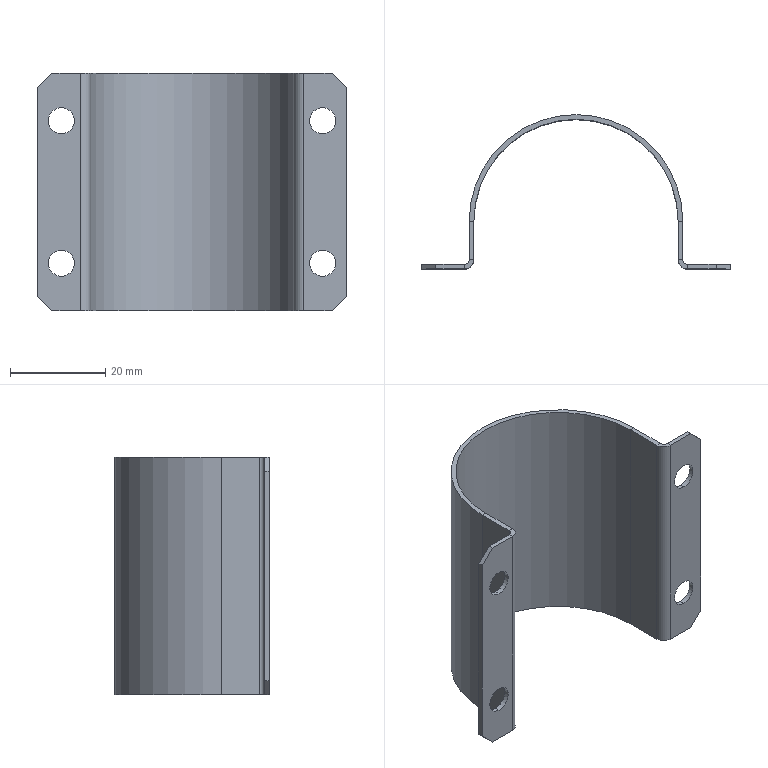Part | STEP file | HXGR200008-05-24 | 1 solid | 42 faces | box 65 x 32.5 x 50 mm | volume 5278 mm3 | plane 28 | cylinder 14 | commonest cylinder face diameters 5.5 x8 2 x2 4 x2 43 x1 45 x1
STEP:
#1=CARTESIAN_POINT('',(-27.5,-10.,-42.75));
#2=VERTEX_POINT('',#1);
#3=CARTESIAN_POINT('',(-27.5,-10.,-37.25));
#4=VERTEX_POINT('',#3);
#5=CARTESIAN_POINT('',(-27.5,-10.,-40.));
#6=DIRECTION('',(0.,1.,0.));
#7=DIRECTION('',(-1.,0.,0.));
#8=AXIS2_PLACEMENT_3D('',#5,#6,#7);
#9=CIRCLE('',#8,2.75);
#10=EDGE_CURVE('',#2,#4,#9,.T.);
#11=ORIENTED_EDGE('',*,*,#10,.F.);
#12=CARTESIAN_POINT('',(-27.5,-9.,-42.75));
#13=VERTEX_POINT('',#12);
#14=CARTESIAN_POINT('',(-27.5,-9.,-42.75));
#15=DIRECTION('',(0.,1.,0.));
#16=VECTOR('',#15,1000.);
#17=LINE('',#14,#16);
#18=EDGE_CURVE('',#2,#13,#17,.T.);
#19=ORIENTED_EDGE('',*,*,#18,.T.);
#20=CARTESIAN_POINT('',(-27.5,-9.,-37.25));
#21=VERTEX_POINT('',#20);
#22=CARTESIAN_POINT('',(-27.5,-9.,-40.));
#23=DIRECTION('',(0.,1.,0.));
#24=DIRECTION('',(0.,0.,1.));
#25=AXIS2_PLACEMENT_3D('',#22,#23,#24);
#26=CIRCLE('',#25,2.75);
#27=EDGE_CURVE('',#13,#21,#26,.T.);
#28=ORIENTED_EDGE('',*,*,#27,.T.);
#29=CARTESIAN_POINT('',(-27.5,-9.,-37.25));
#30=DIRECTION('',(0.,1.,0.));
#31=VECTOR('',#30,1000.);
#32=LINE('',#29,#31);
#33=EDGE_CURVE('',#4,#21,#32,.T.);
#34=ORIENTED_EDGE('',*,*,#33,.F.);
#35=EDGE_LOOP('',(#11,#19,#28,#34));
#36=FACE_OUTER_BOUND('',#35,.T.);
#37=CARTESIAN_POINT('',(-27.5,-9.,-40.));
#38=DIRECTION('',(0.,1.,0.));
#39=DIRECTION('',(0.,0.,1.));
#40=AXIS2_PLACEMENT_3D('',#37,#38,#39);
#41=CYLINDRICAL_SURFACE('',#40,2.75);
#42=ADVANCED_FACE('',(#36),#41,.F.);
#43=CARTESIAN_POINT('',(-27.5,-10.,-12.75));
#44=VERTEX_POINT('',#43);
#45=CARTESIAN_POINT('',(-27.5,-10.,-7.25));
#46=VERTEX_POINT('',#45);
#47=CARTESIAN_POINT('',(-27.5,-10.,-10.));
#48=DIRECTION('',(0.,1.,0.));
#49=DIRECTION('',(-1.,0.,0.));
#50=AXIS2_PLACEMENT_3D('',#47,#48,#49);
#51=CIRCLE('',#50,2.75);
#52=EDGE_CURVE('',#44,#46,#51,.T.);
#53=ORIENTED_EDGE('',*,*,#52,.F.);
#54=CARTESIAN_POINT('',(-27.5,-9.,-12.75));
#55=VERTEX_POINT('',#54);
#56=CARTESIAN_POINT('',(-27.5,-9.,-12.75));
#57=DIRECTION('',(0.,1.,0.));
#58=VECTOR('',#57,1000.);
#59=LINE('',#56,#58);
#60=EDGE_CURVE('',#44,#55,#59,.T.);
#61=ORIENTED_EDGE('',*,*,#60,.T.);
#62=CARTESIAN_POINT('',(-27.5,-9.,-7.25));
#63=VERTEX_POINT('',#62);
#64=CARTESIAN_POINT('',(-27.5,-9.,-10.));
#65=DIRECTION('',(0.,1.,0.));
#66=DIRECTION('',(0.,0.,1.));
#67=AXIS2_PLACEMENT_3D('',#64,#65,#66);
#68=CIRCLE('',#67,2.75);
#69=EDGE_CURVE('',#55,#63,#68,.T.);
#70=ORIENTED_EDGE('',*,*,#69,.T.);
#71=CARTESIAN_POINT('',(-27.5,-9.,-7.25));
#72=DIRECTION('',(0.,1.,0.));
#73=VECTOR('',#72,1000.);
#74=LINE('',#71,#73);
#75=EDGE_CURVE('',#46,#63,#74,.T.);
#76=ORIENTED_EDGE('',*,*,#75,.F.);
#77=EDGE_LOOP('',(#53,#61,#70,#76));
#78=FACE_OUTER_BOUND('',#77,.T.);
#79=CARTESIAN_POINT('',(-27.5,-9.,-10.));
#80=DIRECTION('',(0.,1.,0.));
#81=DIRECTION('',(0.,0.,1.));
#82=AXIS2_PLACEMENT_3D('',#79,#80,#81);
#83=CYLINDRICAL_SURFACE('',#82,2.75);
#84=ADVANCED_FACE('',(#78),#83,.F.);
#85=CARTESIAN_POINT('',(27.5,-10.,-42.75));
#86=VERTEX_POINT('',#85);
#87=CARTESIAN_POINT('',(27.5,-10.,-37.25));
#88=VERTEX_POINT('',#87);
#89=CARTESIAN_POINT('',(27.5,-10.,-40.));
#90=DIRECTION('',(0.,1.,0.));
#91=DIRECTION('',(-1.,0.,0.));
#92=AXIS2_PLACEMENT_3D('',#89,#90,#91);
#93=CIRCLE('',#92,2.75);
#94=EDGE_CURVE('',#86,#88,#93,.T.);
#95=ORIENTED_EDGE('',*,*,#94,.F.);
#96=CARTESIAN_POINT('',(27.5,-9.,-42.75));
#97=VERTEX_POINT('',#96);
#98=CARTESIAN_POINT('',(27.5,-9.,-42.75));
#99=DIRECTION('',(0.,1.,0.));
#100=VECTOR('',#99,1000.);
#101=LINE('',#98,#100);
#102=EDGE_CURVE('',#86,#97,#101,.T.);
#103=ORIENTED_EDGE('',*,*,#102,.T.);
#104=CARTESIAN_POINT('',(27.5,-9.,-37.25));
#105=VERTEX_POINT('',#104);
#106=CARTESIAN_POINT('',(27.5,-9.,-40.));
#107=DIRECTION('',(0.,1.,0.));
#108=DIRECTION('',(0.,0.,1.));
#109=AXIS2_PLACEMENT_3D('',#106,#107,#108);
#110=CIRCLE('',#109,2.75);
#111=EDGE_CURVE('',#97,#105,#110,.T.);
#112=ORIENTED_EDGE('',*,*,#111,.T.);
#113=CARTESIAN_POINT('',(27.5,-9.,-37.25));
#114=DIRECTION('',(0.,1.,0.));
#115=VECTOR('',#114,1000.);
#116=LINE('',#113,#115);
#117=EDGE_CURVE('',#88,#105,#116,.T.);
#118=ORIENTED_EDGE('',*,*,#117,.F.);
#119=EDGE_LOOP('',(#95,#103,#112,#118));
#120=FACE_OUTER_BOUND('',#119,.T.);
#121=CARTESIAN_POINT('',(27.5,-9.,-40.));
#122=DIRECTION('',(0.,1.,0.));
#123=DIRECTION('',(0.,0.,1.));
#124=AXIS2_PLACEMENT_3D('',#121,#122,#123);
#125=CYLINDRICAL_SURFACE('',#124,2.75);
#126=ADVANCED_FACE('',(#120),#125,.F.);
#127=CARTESIAN_POINT('',(27.5,-10.,-12.75));
#128=VERTEX_POINT('',#127);
#129=CARTESIAN_POINT('',(27.5,-10.,-7.25));
#130=VERTEX_POINT('',#129);
#131=CARTESIAN_POINT('',(27.5,-10.,-10.));
#132=DIRECTION('',(0.,1.,0.));
#133=DIRECTION('',(-1.,0.,0.));
#134=AXIS2_PLACEMENT_3D('',#131,#132,#133);
#135=CIRCLE('',#134,2.75);
#136=EDGE_CURVE('',#128,#130,#135,.T.);
#137=ORIENTED_EDGE('',*,*,#136,.F.);
#138=CARTESIAN_POINT('',(27.5,-9.,-12.75));
#139=VERTEX_POINT('',#138);
#140=CARTESIAN_POINT('',(27.5,-9.,-12.75));
#141=DIRECTION('',(0.,1.,0.));
#142=VECTOR('',#141,1000.);
#143=LINE('',#140,#142);
#144=EDGE_CURVE('',#128,#139,#143,.T.);
#145=ORIENTED_EDGE('',*,*,#144,.T.);
#146=CARTESIAN_POINT('',(27.5,-9.,-7.25));
#147=VERTEX_POINT('',#146);
#148=CARTESIAN_POINT('',(27.5,-9.,-10.));
#149=DIRECTION('',(0.,1.,0.));
#150=DIRECTION('',(0.,0.,1.));
#151=AXIS2_PLACEMENT_3D('',#148,#149,#150);
#152=CIRCLE('',#151,2.75);
#153=EDGE_CURVE('',#139,#147,#152,.T.);
#154=ORIENTED_EDGE('',*,*,#153,.T.);
#155=CARTESIAN_POINT('',(27.5,-9.,-7.25));
#156=DIRECTION('',(0.,1.,0.));
#157=VECTOR('',#156,1000.);
#158=LINE('',#155,#157);
#159=EDGE_CURVE('',#130,#147,#158,.T.);
#160=ORIENTED_EDGE('',*,*,#159,.F.);
#161=EDGE_LOOP('',(#137,#145,#154,#160));
#162=FACE_OUTER_BOUND('',#161,.T.);
#163=CARTESIAN_POINT('',(27.5,-9.,-10.));
#164=DIRECTION('',(0.,1.,0.));
#165=DIRECTION('',(0.,0.,1.));
#166=AXIS2_PLACEMENT_3D('',#163,#164,#165);
#167=CYLINDRICAL_SURFACE('',#166,2.75);
#168=ADVANCED_FACE('',(#162),#167,.F.);
#169=CARTESIAN_POINT('',(21.5,0.,-50.));
#170=VERTEX_POINT('',#169);
#171=CARTESIAN_POINT('',(21.5,-8.,-50.));
#172=VERTEX_POINT('',#171);
#173=CARTESIAN_POINT('',(21.5,0.,-50.));
#174=DIRECTION('',(0.,-1.,0.));
#175=VECTOR('',#174,1000.);
#176=LINE('',#173,#175);
#177=EDGE_CURVE('',#170,#172,#176,.T.);
#178=ORIENTED_EDGE('',*,*,#177,.T.);
#179=CARTESIAN_POINT('',(21.5,-8.,0.));
#180=VERTEX_POINT('',#179);
#181=CARTESIAN_POINT('',(21.5,-8.,-50.));
#182=DIRECTION('',(0.,0.,1.));
#183=VECTOR('',#182,1000.);
#184=LINE('',#181,#183);
#185=EDGE_CURVE('',#172,#180,#184,.T.);
#186=ORIENTED_EDGE('',*,*,#185,.T.);
#187=CARTESIAN_POINT('',(21.5,0.,0.));
#188=VERTEX_POINT('',#187);
#189=CARTESIAN_POINT('',(21.5,0.,0.));
#190=DIRECTION('',(0.,-1.,0.));
#191=VECTOR('',#190,1000.);
#192=LINE('',#189,#191);
#193=EDGE_CURVE('',#188,#180,#192,.T.);
#194=ORIENTED_EDGE('',*,*,#193,.F.);
#195=CARTESIAN_POINT('',(21.5,0.,-50.));
#196=DIRECTION('',(0.,0.,1.));
#197=VECTOR('',#196,1000.);
#198=LINE('',#195,#197);
#199=EDGE_CURVE('',#170,#188,#198,.T.);
#200=ORIENTED_EDGE('',*,*,#199,.F.);
#201=EDGE_LOOP('',(#178,#186,#194,#200));
#202=FACE_OUTER_BOUND('',#201,.T.);
#203=CARTESIAN_POINT('',(21.5,0.,-50.));
#204=DIRECTION('',(-1.,0.,0.));
#205=DIRECTION('',(0.,0.,1.));
#206=AXIS2_PLACEMENT_3D('',#203,#204,#205);
#207=PLANE('',#206);
#208=ADVANCED_FACE('',(#202),#207,.T.);
#209=CARTESIAN_POINT('',(22.5,-8.,-50.));
#210=VERTEX_POINT('',#209);
#211=CARTESIAN_POINT('',(22.5,-8.,0.));
#212=VERTEX_POINT('',#211);
#213=CARTESIAN_POINT('',(22.5,-8.,-50.));
#214=DIRECTION('',(0.,0.,1.));
#215=VECTOR('',#214,1000.);
#216=LINE('',#213,#215);
#217=EDGE_CURVE('',#210,#212,#216,.T.);
#218=ORIENTED_EDGE('',*,*,#217,.F.);
#219=CARTESIAN_POINT('',(22.5,0.,-50.));
#220=VERTEX_POINT('',#219);
#221=CARTESIAN_POINT('',(22.5,0.,-50.));
#222=DIRECTION('',(0.,-1.,0.));
#223=VECTOR('',#222,1000.);
#224=LINE('',#221,#223);
#225=EDGE_CURVE('',#220,#210,#224,.T.);
#226=ORIENTED_EDGE('',*,*,#225,.F.);
#227=CARTESIAN_POINT('',(22.5,0.,0.));
#228=VERTEX_POINT('',#227);
#229=CARTESIAN_POINT('',(22.5,0.,-50.));
#230=DIRECTION('',(0.,0.,1.));
#231=VECTOR('',#230,1000.);
#232=LINE('',#229,#231);
#233=EDGE_CURVE('',#220,#228,#232,.T.);
#234=ORIENTED_EDGE('',*,*,#233,.T.);
#235=CARTESIAN_POINT('',(22.5,0.,0.));
#236=DIRECTION('',(0.,-1.,0.));
#237=VECTOR('',#236,1000.);
#238=LINE('',#235,#237);
#239=EDGE_CURVE('',#228,#212,#238,.T.);
#240=ORIENTED_EDGE('',*,*,#239,.T.);
#241=EDGE_LOOP('',(#218,#226,#234,#240));
#242=FACE_OUTER_BOUND('',#241,.T.);
#243=CARTESIAN_POINT('',(22.5,0.,-50.));
#244=DIRECTION('',(-1.,0.,0.));
#245=DIRECTION('',(0.,0.,1.));
#246=AXIS2_PLACEMENT_3D('',#243,#244,#245);
#247=PLANE('',#246);
#248=ADVANCED_FACE('',(#242),#247,.F.);
#249=ORIENTED_EDGE('',*,*,#225,.T.);
#250=CARTESIAN_POINT('',(22.5,-8.,-50.));
#251=DIRECTION('',(-1.,0.,0.));
#252=VECTOR('',#251,1000.);
#253=LINE('',#250,#252);
#254=EDGE_CURVE('',#210,#172,#253,.T.);
#255=ORIENTED_EDGE('',*,*,#254,.T.);
#256=ORIENTED_EDGE('',*,*,#177,.F.);
#257=CARTESIAN_POINT('',(21.5,0.,-50.));
#258=DIRECTION('',(1.,0.,0.));
#259=VECTOR('',#258,1000.);
#260=LINE('',#257,#259);
#261=EDGE_CURVE('',#170,#220,#260,.T.);
#262=ORIENTED_EDGE('',*,*,#261,.T.);
#263=EDGE_LOOP('',(#249,#255,#256,#262));
#264=FACE_OUTER_BOUND('',#263,.T.);
#265=CARTESIAN_POINT('',(0.,0.,-50.));
#266=DIRECTION('',(0.,0.,-1.));
#267=DIRECTION('',(-1.,0.,0.));
#268=AXIS2_PLACEMENT_3D('',#265,#266,#267);
#269=PLANE('',#268);
#270=ADVANCED_FACE('',(#264),#269,.T.);
#271=CARTESIAN_POINT('',(-21.5,-8.,0.));
#272=VERTEX_POINT('',#271);
#273=CARTESIAN_POINT('',(-21.5,0.,0.));
#274=VERTEX_POINT('',#273);
#275=CARTESIAN_POINT('',(-21.5,0.,0.));
#276=DIRECTION('',(0.,1.,0.));
#277=VECTOR('',#276,1000.);
#278=LINE('',#275,#277);
#279=EDGE_CURVE('',#272,#274,#278,.T.);
#280=ORIENTED_EDGE('',*,*,#279,.F.);
#281=CARTESIAN_POINT('',(-21.5,-8.,-50.));
#282=VERTEX_POINT('',#281);
#283=CARTESIAN_POINT('',(-21.5,-8.,0.));
#284=DIRECTION('',(0.,0.,-1.));
#285=VECTOR('',#284,1000.);
#286=LINE('',#283,#285);
#287=EDGE_CURVE('',#272,#282,#286,.T.);
#288=ORIENTED_EDGE('',*,*,#287,.T.);
#289=CARTESIAN_POINT('',(-21.5,0.,-50.));
#290=VERTEX_POINT('',#289);
#291=CARTESIAN_POINT('',(-21.5,0.,-50.));
#292=DIRECTION('',(0.,1.,0.));
#293=VECTOR('',#292,1000.);
#294=LINE('',#291,#293);
#295=EDGE_CURVE('',#282,#290,#294,.T.);
#296=ORIENTED_EDGE('',*,*,#295,.T.);
#297=CARTESIAN_POINT('',(-21.5,0.,-50.));
#298=DIRECTION('',(0.,0.,1.));
#299=VECTOR('',#298,1000.);
#300=LINE('',#297,#299);
#301=EDGE_CURVE('',#290,#274,#300,.T.);
#302=ORIENTED_EDGE('',*,*,#301,.T.);
#303=EDGE_LOOP('',(#280,#288,#296,#302));
#304=FACE_OUTER_BOUND('',#303,.T.);
#305=CARTESIAN_POINT('',(-21.5,0.,-50.));
#306=DIRECTION('',(1.,0.,0.));
#307=DIRECTION('',(0.,0.,-1.));
#308=AXIS2_PLACEMENT_3D('',#305,#306,#307);
#309=PLANE('',#308);
#310=ADVANCED_FACE('',(#304),#309,.T.);
#311=CARTESIAN_POINT('',(-22.5,-8.,0.));
#312=VERTEX_POINT('',#311);
#313=CARTESIAN_POINT('',(-22.5,-8.,-50.));
#314=VERTEX_POINT('',#313);
#315=CARTESIAN_POINT('',(-22.5,-8.,0.));
#316=DIRECTION('',(0.,0.,-1.));
#317=VECTOR('',#316,1000.);
#318=LINE('',#315,#317);
#319=EDGE_CURVE('',#312,#314,#318,.T.);
#320=ORIENTED_EDGE('',*,*,#319,.F.);
#321=CARTESIAN_POINT('',(-22.5,0.,0.));
#322=VERTEX_POINT('',#321);
#323=CARTESIAN_POINT('',(-22.5,0.,0.));
#324=DIRECTION('',(0.,1.,0.));
#325=VECTOR('',#324,1000.);
#326=LINE('',#323,#325);
#327=EDGE_CURVE('',#312,#322,#326,.T.);
#328=ORIENTED_EDGE('',*,*,#327,.T.);
#329=CARTESIAN_POINT('',(-22.5,0.,-50.));
#330=VERTEX_POINT('',#329);
#331=CARTESIAN_POINT('',(-22.5,0.,-50.));
#332=DIRECTION('',(0.,0.,1.));
#333=VECTOR('',#332,1000.);
#334=LINE('',#331,#333);
#335=EDGE_CURVE('',#330,#322,#334,.T.);
#336=ORIENTED_EDGE('',*,*,#335,.F.);
#337=CARTESIAN_POINT('',(-22.5,0.,-50.));
#338=DIRECTION('',(0.,1.,0.));
#339=VECTOR('',#338,1000.);
#340=LINE('',#337,#339);
#341=EDGE_CURVE('',#314,#330,#340,.T.);
#342=ORIENTED_EDGE('',*,*,#341,.F.);
#343=EDGE_LOOP('',(#320,#328,#336,#342));
#344=FACE_OUTER_BOUND('',#343,.T.);
#345=CARTESIAN_POINT('',(-22.5,0.,-50.));
#346=DIRECTION('',(1.,0.,0.));
#347=DIRECTION('',(0.,0.,-1.));
#348=AXIS2_PLACEMENT_3D('',#345,#346,#347);
#349=PLANE('',#348);
#350=ADVANCED_FACE('',(#344),#349,.F.);
#351=CARTESIAN_POINT('',(-22.5,-8.,0.));
#352=DIRECTION('',(1.,0.,0.));
#353=VECTOR('',#352,1000.);
#354=LINE('',#351,#353);
#355=EDGE_CURVE('',#312,#272,#354,.T.);
#356=ORIENTED_EDGE('',*,*,#355,.T.);
#357=ORIENTED_EDGE('',*,*,#279,.T.);
#358=CARTESIAN_POINT('',(-21.5,0.,0.));
#359=DIRECTION('',(-1.,0.,0.));
#360=VECTOR('',#359,1000.);
#361=LINE('',#358,#360);
#362=EDGE_CURVE('',#274,#322,#361,.T.);
#363=ORIENTED_EDGE('',*,*,#362,.T.);
#364=ORIENTED_EDGE('',*,*,#327,.F.);
#365=EDGE_LOOP('',(#356,#357,#363,#364));
#366=FACE_OUTER_BOUND('',#365,.T.);
#367=CARTESIAN_POINT('',(0.,0.,0.));
#368=DIRECTION('',(0.,0.,-1.));
#369=DIRECTION('',(-1.,0.,0.));
#370=AXIS2_PLACEMENT_3D('',#367,#368,#369);
#371=PLANE('',#370);
#372=ADVANCED_FACE('',(#366),#371,.F.);
#373=CARTESIAN_POINT('',(-22.5,0.,-50.));
#374=DIRECTION('',(1.,0.,0.));
#375=VECTOR('',#374,1000.);
#376=LINE('',#373,#375);
#377=EDGE_CURVE('',#330,#290,#376,.T.);
#378=ORIENTED_EDGE('',*,*,#377,.F.);
#379=CARTESIAN_POINT('',(0.,0.,-50.));
#380=DIRECTION('',(0.,0.,-1.));
#381=DIRECTION('',(1.,0.,0.));
#382=AXIS2_PLACEMENT_3D('',#379,#380,#381);
#383=CIRCLE('',#382,22.5);
#384=EDGE_CURVE('',#330,#220,#383,.T.);
#385=ORIENTED_EDGE('',*,*,#384,.T.);
#386=ORIENTED_EDGE('',*,*,#261,.F.);
#387=CARTESIAN_POINT('',(0.,0.,-50.));
#388=DIRECTION('',(0.,0.,-1.));
#389=DIRECTION('',(1.,0.,0.));
#390=AXIS2_PLACEMENT_3D('',#387,#388,#389);
#391=CIRCLE('',#390,21.5);
#392=EDGE_CURVE('',#290,#170,#391,.T.);
#393=ORIENTED_EDGE('',*,*,#392,.F.);
#394=EDGE_LOOP('',(#378,#385,#386,#393));
#395=FACE_OUTER_BOUND('',#394,.T.);
#396=CARTESIAN_POINT('',(-22.5,0.,-50.));
#397=DIRECTION('',(0.,0.,-1.));
#398=DIRECTION('',(-1.,0.,0.));
#399=AXIS2_PLACEMENT_3D('',#396,#397,#398);
#400=PLANE('',#399);
#401=ADVANCED_FACE('',(#395),#400,.T.);
#402=CARTESIAN_POINT('',(-22.5,-8.,-50.));
#403=DIRECTION('',(1.,0.,0.));
#404=VECTOR('',#403,1000.);
#405=LINE('',#402,#404);
#406=EDGE_CURVE('',#314,#282,#405,.T.);
#407=ORIENTED_EDGE('',*,*,#406,.F.);
#408=ORIENTED_EDGE('',*,*,#341,.T.);
#409=ORIENTED_EDGE('',*,*,#377,.T.);
#410=ORIENTED_EDGE('',*,*,#295,.F.);
#411=EDGE_LOOP('',(#407,#408,#409,#410));
#412=FACE_OUTER_BOUND('',#411,.T.);
#413=CARTESIAN_POINT('',(21.5,0.,-50.));
#414=DIRECTION('',(0.,0.,-1.));
#415=DIRECTION('',(-1.,0.,0.));
#416=AXIS2_PLACEMENT_3D('',#413,#414,#415);
#417=PLANE('',#416);
#418=ADVANCED_FACE('',(#412),#417,.T.);
#419=CARTESIAN_POINT('',(22.5,0.,0.));
#420=DIRECTION('',(-1.,0.,0.));
#421=VECTOR('',#420,1000.);
#422=LINE('',#419,#421);
#423=EDGE_CURVE('',#228,#188,#422,.T.);
#424=ORIENTED_EDGE('',*,*,#423,.F.);
#425=CARTESIAN_POINT('',(0.,0.,0.));
#426=DIRECTION('',(0.,0.,-1.));
#427=DIRECTION('',(1.,0.,0.));
#428=AXIS2_PLACEMENT_3D('',#425,#426,#427);
#429=CIRCLE('',#428,22.5);
#430=EDGE_CURVE('',#322,#228,#429,.T.);
#431=ORIENTED_EDGE('',*,*,#430,.F.);
#432=ORIENTED_EDGE('',*,*,#362,.F.);
#433=CARTESIAN_POINT('',(0.,0.,0.));
#434=DIRECTION('',(0.,0.,-1.));
#435=DIRECTION('',(1.,0.,0.));
#436=AXIS2_PLACEMENT_3D('',#433,#434,#435);
#437=CIRCLE('',#436,21.5);
#438=EDGE_CURVE('',#274,#188,#437,.T.);
#439=ORIENTED_EDGE('',*,*,#438,.T.);
#440=EDGE_LOOP('',(#424,#431,#432,#439));
#441=FACE_OUTER_BOUND('',#440,.T.);
#442=CARTESIAN_POINT('',(22.5,0.,0.));
#443=DIRECTION('',(0.,0.,1.));
#444=DIRECTION('',(1.,0.,0.));
#445=AXIS2_PLACEMENT_3D('',#442,#443,#444);
#446=PLANE('',#445);
#447=ADVANCED_FACE('',(#441),#446,.T.);
#448=CARTESIAN_POINT('',(22.5,-8.,0.));
#449=DIRECTION('',(-1.,0.,0.));
#450=VECTOR('',#449,1000.);
#451=LINE('',#448,#450);
#452=EDGE_CURVE('',#212,#180,#451,.T.);
#453=ORIENTED_EDGE('',*,*,#452,.F.);
#454=ORIENTED_EDGE('',*,*,#239,.F.);
#455=ORIENTED_EDGE('',*,*,#423,.T.);
#456=ORIENTED_EDGE('',*,*,#193,.T.);
#457=EDGE_LOOP('',(#453,#454,#455,#456));
#458=FACE_OUTER_BOUND('',#457,.T.);
#459=CARTESIAN_POINT('',(-21.5,0.,0.));
#460=DIRECTION('',(0.,0.,1.));
#461=DIRECTION('',(1.,0.,0.));
#462=AXIS2_PLACEMENT_3D('',#459,#460,#461);
#463=PLANE('',#462);
#464=ADVANCED_FACE('',(#458),#463,.T.);
#465=ORIENTED_EDGE('',*,*,#438,.F.);
#466=ORIENTED_EDGE('',*,*,#301,.F.);
#467=ORIENTED_EDGE('',*,*,#392,.T.);
#468=ORIENTED_EDGE('',*,*,#199,.T.);
#469=EDGE_LOOP('',(#465,#466,#467,#468));
#470=FACE_OUTER_BOUND('',#469,.T.);
#471=CARTESIAN_POINT('',(0.,0.,-50.));
#472=DIRECTION('',(0.,0.,1.));
#473=DIRECTION('',(1.,0.,0.));
#474=AXIS2_PLACEMENT_3D('',#471,#472,#473);
#475=CYLINDRICAL_SURFACE('',#474,21.5);
#476=ADVANCED_FACE('',(#470),#475,.F.);
#477=ORIENTED_EDGE('',*,*,#430,.T.);
#478=ORIENTED_EDGE('',*,*,#233,.F.);
#479=ORIENTED_EDGE('',*,*,#384,.F.);
#480=ORIENTED_EDGE('',*,*,#335,.T.);
#481=EDGE_LOOP('',(#477,#478,#479,#480));
#482=FACE_OUTER_BOUND('',#481,.T.);
#483=CARTESIAN_POINT('',(0.,0.,-50.));
#484=DIRECTION('',(0.,0.,1.));
#485=DIRECTION('',(1.,0.,0.));
#486=AXIS2_PLACEMENT_3D('',#483,#484,#485);
#487=CYLINDRICAL_SURFACE('',#486,22.5);
#488=ADVANCED_FACE('',(#482),#487,.T.);
#489=CARTESIAN_POINT('',(-23.5,-9.,-50.));
#490=VERTEX_POINT('',#489);
#491=CARTESIAN_POINT('',(-23.5,-10.,-50.));
#492=VERTEX_POINT('',#491);
#493=CARTESIAN_POINT('',(-23.5,-10.,-50.));
#494=DIRECTION('',(0.,-1.,0.));
#495=VECTOR('',#494,1000.);
#496=LINE('',#493,#495);
#497=EDGE_CURVE('',#490,#492,#496,.T.);
#498=ORIENTED_EDGE('',*,*,#497,.F.);
#499=CARTESIAN_POINT('',(-23.5,-8.,-50.));
#500=DIRECTION('',(0.,0.,-1.));
#501=DIRECTION('',(1.,0.,0.));
#502=AXIS2_PLACEMENT_3D('',#499,#500,#501);
#503=CIRCLE('',#502,1.);
#504=EDGE_CURVE('',#314,#490,#503,.T.);
#505=ORIENTED_EDGE('',*,*,#504,.F.);
#506=ORIENTED_EDGE('',*,*,#406,.T.);
#507=CARTESIAN_POINT('',(-23.5,-8.,-50.));
#508=DIRECTION('',(0.,0.,-1.));
#509=DIRECTION('',(1.,0.,0.));
#510=AXIS2_PLACEMENT_3D('',#507,#508,#509);
#511=CIRCLE('',#510,2.);
#512=EDGE_CURVE('',#282,#492,#511,.T.);
#513=ORIENTED_EDGE('',*,*,#512,.T.);
#514=EDGE_LOOP('',(#498,#505,#506,#513));
#515=FACE_OUTER_BOUND('',#514,.T.);
#516=CARTESIAN_POINT('',(-23.5,-8.,-50.));
#517=DIRECTION('',(0.,0.,-1.));
#518=DIRECTION('',(-1.,0.,0.));
#519=AXIS2_PLACEMENT_3D('',#516,#517,#518);
#520=PLANE('',#519);
#521=ADVANCED_FACE('',(#515),#520,.T.);
#522=CARTESIAN_POINT('',(-23.5,-9.,0.));
#523=VERTEX_POINT('',#522);
#524=CARTESIAN_POINT('',(-23.5,-8.,0.));
#525=DIRECTION('',(0.,0.,1.));
#526=DIRECTION('',(1.,0.,0.));
#527=AXIS2_PLACEMENT_3D('',#524,#525,#526);
#528=CIRCLE('',#527,1.);
#529=EDGE_CURVE('',#523,#312,#528,.T.);
#530=ORIENTED_EDGE('',*,*,#529,.F.);
#531=CARTESIAN_POINT('',(-23.5,-10.,0.));
#532=VERTEX_POINT('',#531);
#533=CARTESIAN_POINT('',(-23.5,-9.,0.));
#534=DIRECTION('',(0.,-1.,0.));
#535=VECTOR('',#534,1000.);
#536=LINE('',#533,#535);
#537=EDGE_CURVE('',#523,#532,#536,.T.);
#538=ORIENTED_EDGE('',*,*,#537,.T.);
#539=CARTESIAN_POINT('',(-23.5,-8.,0.));
#540=DIRECTION('',(0.,0.,1.));
#541=DIRECTION('',(1.,0.,0.));
#542=AXIS2_PLACEMENT_3D('',#539,#540,#541);
#543=CIRCLE('',#542,2.);
#544=EDGE_CURVE('',#532,#272,#543,.T.);
#545=ORIENTED_EDGE('',*,*,#544,.T.);
#546=ORIENTED_EDGE('',*,*,#355,.F.);
#547=EDGE_LOOP('',(#530,#538,#545,#546));
#548=FACE_OUTER_BOUND('',#547,.T.);
#549=CARTESIAN_POINT('',(-23.5,-8.,0.));
#550=DIRECTION('',(0.,0.,-1.));
#551=DIRECTION('',(-1.,0.,0.));
#552=AXIS2_PLACEMENT_3D('',#549,#550,#551);
#553=PLANE('',#552);
#554=ADVANCED_FACE('',(#548),#553,.F.);
#555=ORIENTED_EDGE('',*,*,#287,.F.);
#556=ORIENTED_EDGE('',*,*,#544,.F.);
#557=CARTESIAN_POINT('',(-23.5,-10.,-50.));
#558=DIRECTION('',(0.,0.,-1.));
#559=VECTOR('',#558,1000.);
#560=LINE('',#557,#559);
#561=EDGE_CURVE('',#532,#492,#560,.T.);
#562=ORIENTED_EDGE('',*,*,#561,.T.);
#563=ORIENTED_EDGE('',*,*,#512,.F.);
#564=EDGE_LOOP('',(#555,#556,#562,#563));
#565=FACE_OUTER_BOUND('',#564,.T.);
#566=CARTESIAN_POINT('',(-23.5,-8.,0.));
#567=DIRECTION('',(0.,0.,1.));
#568=DIRECTION('',(0.,-1.,0.));
#569=AXIS2_PLACEMENT_3D('',#566,#567,#568);
#570=CYLINDRICAL_SURFACE('',#569,2.);
#571=ADVANCED_FACE('',(#565),#570,.T.);
#572=ORIENTED_EDGE('',*,*,#319,.T.);
#573=ORIENTED_EDGE('',*,*,#504,.T.);
#574=CARTESIAN_POINT('',(-23.5,-9.,-50.));
#575=DIRECTION('',(0.,0.,1.));
#576=VECTOR('',#575,1000.);
#577=LINE('',#574,#576);
#578=EDGE_CURVE('',#490,#523,#577,.T.);
#579=ORIENTED_EDGE('',*,*,#578,.T.);
#580=ORIENTED_EDGE('',*,*,#529,.T.);
#581=EDGE_LOOP('',(#572,#573,#579,#580));
#582=FACE_OUTER_BOUND('',#581,.T.);
#583=CARTESIAN_POINT('',(-23.5,-8.,0.));
#584=DIRECTION('',(0.,0.,1.));
#585=DIRECTION('',(0.,-1.,0.));
#586=AXIS2_PLACEMENT_3D('',#583,#584,#585);
#587=CYLINDRICAL_SURFACE('',#586,1.);
#588=ADVANCED_FACE('',(#582),#587,.F.);
#589=CARTESIAN_POINT('',(-29.5,-10.,-50.));
#590=VERTEX_POINT('',#589);
#591=CARTESIAN_POINT('',(0.,-10.,-50.));
#592=DIRECTION('',(1.,0.,0.));
#593=VECTOR('',#592,1000.);
#594=LINE('',#591,#593);
#595=EDGE_CURVE('',#590,#492,#594,.T.);
#596=ORIENTED_EDGE('',*,*,#595,.F.);
#597=CARTESIAN_POINT('',(-29.5,-9.,-50.));
#598=VERTEX_POINT('',#597);
#599=CARTESIAN_POINT('',(-29.5,-10.,-50.));
#600=DIRECTION('',(0.,1.,0.));
#601=VECTOR('',#600,1000.);
#602=LINE('',#599,#601);
#603=EDGE_CURVE('',#590,#598,#602,.T.);
#604=ORIENTED_EDGE('',*,*,#603,.T.);
#605=CARTESIAN_POINT('',(-22.5,-9.,-50.));
#606=DIRECTION('',(1.,0.,0.));
#607=VECTOR('',#606,1000.);
#608=LINE('',#605,#607);
#609=EDGE_CURVE('',#598,#490,#608,.T.);
#610=ORIENTED_EDGE('',*,*,#609,.T.);
#611=ORIENTED_EDGE('',*,*,#497,.T.);
#612=EDGE_LOOP('',(#596,#604,#610,#611));
#613=FACE_OUTER_BOUND('',#612,.T.);
#614=CARTESIAN_POINT('',(-22.5,-10.,-50.));
#615=DIRECTION('',(0.,0.,1.));
#616=DIRECTION('',(1.,0.,0.));
#617=AXIS2_PLACEMENT_3D('',#614,#615,#616);
#618=PLANE('',#617);
#619=ADVANCED_FACE('',(#613),#618,.F.);
#620=CARTESIAN_POINT('',(-29.5,-9.,0.));
#621=VERTEX_POINT('',#620);
#622=CARTESIAN_POINT('',(-32.5,-9.,0.));
#623=DIRECTION('',(-1.,0.,0.));
#624=VECTOR('',#623,1000.);
#625=LINE('',#622,#624);
#626=EDGE_CURVE('',#523,#621,#625,.T.);
#627=ORIENTED_EDGE('',*,*,#626,.T.);
#628=CARTESIAN_POINT('',(-29.5,-10.,0.));
#629=VERTEX_POINT('',#628);
#630=CARTESIAN_POINT('',(-29.5,-10.,0.));
#631=DIRECTION('',(0.,-1.,0.));
#632=VECTOR('',#631,1000.);
#633=LINE('',#630,#632);
#634=EDGE_CURVE('',#621,#629,#633,.T.);
#635=ORIENTED_EDGE('',*,*,#634,.T.);
#636=CARTESIAN_POINT('',(0.,-10.,0.));
#637=DIRECTION('',(-1.,0.,0.));
#638=VECTOR('',#637,1000.);
#639=LINE('',#636,#638);
#640=EDGE_CURVE('',#532,#629,#639,.T.);
#641=ORIENTED_EDGE('',*,*,#640,.F.);
#642=ORIENTED_EDGE('',*,*,#537,.F.);
#643=EDGE_LOOP('',(#627,#635,#641,#642));
#644=FACE_OUTER_BOUND('',#643,.T.);
#645=CARTESIAN_POINT('',(-32.5,-10.,0.));
#646=DIRECTION('',(0.,0.,-1.));
#647=DIRECTION('',(-1.,0.,0.));
#648=AXIS2_PLACEMENT_3D('',#645,#646,#647);
#649=PLANE('',#648);
#650=ADVANCED_FACE('',(#644),#649,.F.);
#651=CARTESIAN_POINT('',(-27.5,-10.,-40.));
#652=DIRECTION('',(0.,1.,0.));
#653=DIRECTION('',(-1.,0.,0.));
#654=AXIS2_PLACEMENT_3D('',#651,#652,#653);
#655=CIRCLE('',#654,2.75);
#656=EDGE_CURVE('',#4,#2,#655,.T.);
#657=ORIENTED_EDGE('',*,*,#656,.T.);
#658=ORIENTED_EDGE('',*,*,#10,.T.);
#659=EDGE_LOOP('',(#657,#658));
#660=FACE_BOUND('',#659,.T.);
#661=CARTESIAN_POINT('',(-27.5,-10.,-10.));
#662=DIRECTION('',(0.,1.,0.));
#663=DIRECTION('',(-1.,0.,0.));
#664=AXIS2_PLACEMENT_3D('',#661,#662,#663);
#665=CIRCLE('',#664,2.75);
#666=EDGE_CURVE('',#46,#44,#665,.T.);
#667=ORIENTED_EDGE('',*,*,#666,.T.);
#668=ORIENTED_EDGE('',*,*,#52,.T.);
#669=EDGE_LOOP('',(#667,#668));
#670=FACE_BOUND('',#669,.T.);
#671=CARTESIAN_POINT('',(-32.5,-10.,-3.));
#672=VERTEX_POINT('',#671);
#673=CARTESIAN_POINT('',(-32.5,-10.,-47.));
#674=VERTEX_POINT('',#673);
#675=CARTESIAN_POINT('',(-32.5,-10.,0.));
#676=DIRECTION('',(0.,0.,-1.));
#677=VECTOR('',#676,1000.);
#678=LINE('',#675,#677);
#679=EDGE_CURVE('',#672,#674,#678,.T.);
#680=ORIENTED_EDGE('',*,*,#679,.T.);
#681=CARTESIAN_POINT('',(-29.5,-10.,-50.));
#682=DIRECTION('',(0.7071,0.,-0.7071));
#683=VECTOR('',#682,1000.);
#684=LINE('',#681,#683);
#685=EDGE_CURVE('',#674,#590,#684,.T.);
#686=ORIENTED_EDGE('',*,*,#685,.T.);
#687=ORIENTED_EDGE('',*,*,#595,.T.);
#688=ORIENTED_EDGE('',*,*,#561,.F.);
#689=ORIENTED_EDGE('',*,*,#640,.T.);
#690=CARTESIAN_POINT('',(-32.5,-10.,-3.));
#691=DIRECTION('',(-0.7071,0.,-0.7071));
#692=VECTOR('',#691,1000.);
#693=LINE('',#690,#692);
#694=EDGE_CURVE('',#629,#672,#693,.T.);
#695=ORIENTED_EDGE('',*,*,#694,.T.);
#696=EDGE_LOOP('',(#680,#686,#687,#688,#689,#695));
#697=FACE_OUTER_BOUND('',#696,.T.);
#698=CARTESIAN_POINT('',(0.,-10.,0.));
#699=DIRECTION('',(0.,1.,0.));
#700=DIRECTION('',(-1.,0.,0.));
#701=AXIS2_PLACEMENT_3D('',#698,#699,#700);
#702=PLANE('',#701);
#703=ADVANCED_FACE('',(#660,#670,#697),#702,.F.);
#704=CARTESIAN_POINT('',(-27.5,-9.,-40.));
#705=DIRECTION('',(0.,1.,0.));
#706=DIRECTION('',(0.,0.,1.));
#707=AXIS2_PLACEMENT_3D('',#704,#705,#706);
#708=CIRCLE('',#707,2.75);
#709=EDGE_CURVE('',#21,#13,#708,.T.);
#710=ORIENTED_EDGE('',*,*,#709,.F.);
#711=ORIENTED_EDGE('',*,*,#27,.F.);
#712=EDGE_LOOP('',(#710,#711));
#713=FACE_BOUND('',#712,.T.);
#714=CARTESIAN_POINT('',(-27.5,-9.,-10.));
#715=DIRECTION('',(0.,1.,0.));
#716=DIRECTION('',(0.,0.,1.));
#717=AXIS2_PLACEMENT_3D('',#714,#715,#716);
#718=CIRCLE('',#717,2.75);
#719=EDGE_CURVE('',#63,#55,#718,.T.);
#720=ORIENTED_EDGE('',*,*,#719,.F.);
#721=ORIENTED_EDGE('',*,*,#69,.F.);
#722=EDGE_LOOP('',(#720,#721));
#723=FACE_BOUND('',#722,.T.);
#724=ORIENTED_EDGE('',*,*,#609,.F.);
#725=CARTESIAN_POINT('',(-32.5,-9.,-47.));
#726=VERTEX_POINT('',#725);
#727=CARTESIAN_POINT('',(-39.75,-9.,-39.75));
#728=DIRECTION('',(-0.7071,0.,0.7071));
#729=VECTOR('',#728,1000.);
#730=LINE('',#727,#729);
#731=EDGE_CURVE('',#598,#726,#730,.T.);
#732=ORIENTED_EDGE('',*,*,#731,.T.);
#733=CARTESIAN_POINT('',(-32.5,-9.,-3.));
#734=VERTEX_POINT('',#733);
#735=CARTESIAN_POINT('',(-32.5,-9.,-50.));
#736=DIRECTION('',(0.,0.,-1.));
#737=VECTOR('',#736,1000.);
#738=LINE('',#735,#737);
#739=EDGE_CURVE('',#734,#726,#738,.T.);
#740=ORIENTED_EDGE('',*,*,#739,.F.);
#741=CARTESIAN_POINT('',(-14.75,-9.,14.75));
#742=DIRECTION('',(0.7071,0.,0.7071));
#743=VECTOR('',#742,1000.);
#744=LINE('',#741,#743);
#745=EDGE_CURVE('',#734,#621,#744,.T.);
#746=ORIENTED_EDGE('',*,*,#745,.T.);
#747=ORIENTED_EDGE('',*,*,#626,.F.);
#748=ORIENTED_EDGE('',*,*,#578,.F.);
#749=EDGE_LOOP('',(#724,#732,#740,#746,#747,#748));
#750=FACE_OUTER_BOUND('',#749,.T.);
#751=CARTESIAN_POINT('',(0.,-9.,0.));
#752=DIRECTION('',(0.,1.,0.));
#753=DIRECTION('',(-1.,0.,0.));
#754=AXIS2_PLACEMENT_3D('',#751,#752,#753);
#755=PLANE('',#754);
#756=ADVANCED_FACE('',(#713,#723,#750),#755,.T.);
#757=ORIENTED_EDGE('',*,*,#739,.T.);
#758=CARTESIAN_POINT('',(-32.5,-10.,-47.));
#759=DIRECTION('',(0.,-1.,0.));
#760=VECTOR('',#759,1000.);
#761=LINE('',#758,#760);
#762=EDGE_CURVE('',#726,#674,#761,.T.);
#763=ORIENTED_EDGE('',*,*,#762,.T.);
#764=ORIENTED_EDGE('',*,*,#679,.F.);
#765=CARTESIAN_POINT('',(-32.5,-10.,-3.));
#766=DIRECTION('',(0.,1.,0.));
#767=VECTOR('',#766,1000.);
#768=LINE('',#765,#767);
#769=EDGE_CURVE('',#672,#734,#768,.T.);
#770=ORIENTED_EDGE('',*,*,#769,.T.);
#771=EDGE_LOOP('',(#757,#763,#764,#770));
#772=FACE_OUTER_BOUND('',#771,.T.);
#773=CARTESIAN_POINT('',(-32.5,-10.,-50.));
#774=DIRECTION('',(1.,0.,0.));
#775=DIRECTION('',(0.,1.,0.));
#776=AXIS2_PLACEMENT_3D('',#773,#774,#775);
#777=PLANE('',#776);
#778=ADVANCED_FACE('',(#772),#777,.F.);
#779=CARTESIAN_POINT('',(23.5,-9.,0.));
#780=VERTEX_POINT('',#779);
#781=CARTESIAN_POINT('',(23.5,-10.,0.));
#782=VERTEX_POINT('',#781);
#783=CARTESIAN_POINT('',(23.5,-10.,0.));
#784=DIRECTION('',(0.,-1.,0.));
#785=VECTOR('',#784,1000.);
#786=LINE('',#783,#785);
#787=EDGE_CURVE('',#780,#782,#786,.T.);
#788=ORIENTED_EDGE('',*,*,#787,.F.);
#789=CARTESIAN_POINT('',(23.5,-8.,0.));
#790=DIRECTION('',(0.,0.,1.));
#791=DIRECTION('',(-1.,0.,0.));
#792=AXIS2_PLACEMENT_3D('',#789,#790,#791);
#793=CIRCLE('',#792,1.);
#794=EDGE_CURVE('',#212,#780,#793,.T.);
#795=ORIENTED_EDGE('',*,*,#794,.F.);
#796=ORIENTED_EDGE('',*,*,#452,.T.);
#797=CARTESIAN_POINT('',(23.5,-8.,0.));
#798=DIRECTION('',(0.,0.,1.));
#799=DIRECTION('',(-1.,0.,0.));
#800=AXIS2_PLACEMENT_3D('',#797,#798,#799);
#801=CIRCLE('',#800,2.);
#802=EDGE_CURVE('',#180,#782,#801,.T.);
#803=ORIENTED_EDGE('',*,*,#802,.T.);
#804=EDGE_LOOP('',(#788,#795,#796,#803));
#805=FACE_OUTER_BOUND('',#804,.T.);
#806=CARTESIAN_POINT('',(23.5,-8.,0.));
#807=DIRECTION('',(0.,0.,1.));
#808=DIRECTION('',(1.,0.,0.));
#809=AXIS2_PLACEMENT_3D('',#806,#807,#808);
#810=PLANE('',#809);
#811=ADVANCED_FACE('',(#805),#810,.T.);
#812=CARTESIAN_POINT('',(23.5,-9.,-50.));
#813=VERTEX_POINT('',#812);
#814=CARTESIAN_POINT('',(23.5,-8.,-50.));
#815=DIRECTION('',(0.,0.,-1.));
#816=DIRECTION('',(-1.,0.,0.));
#817=AXIS2_PLACEMENT_3D('',#814,#815,#816);
#818=CIRCLE('',#817,1.);
#819=EDGE_CURVE('',#813,#210,#818,.T.);
#820=ORIENTED_EDGE('',*,*,#819,.F.);
#821=CARTESIAN_POINT('',(23.5,-10.,-50.));
#822=VERTEX_POINT('',#821);
#823=CARTESIAN_POINT('',(23.5,-9.,-50.));
#824=DIRECTION('',(0.,-1.,0.));
#825=VECTOR('',#824,1000.);
#826=LINE('',#823,#825);
#827=EDGE_CURVE('',#813,#822,#826,.T.);
#828=ORIENTED_EDGE('',*,*,#827,.T.);
#829=CARTESIAN_POINT('',(23.5,-8.,-50.));
#830=DIRECTION('',(0.,0.,-1.));
#831=DIRECTION('',(-1.,0.,0.));
#832=AXIS2_PLACEMENT_3D('',#829,#830,#831);
#833=CIRCLE('',#832,2.);
#834=EDGE_CURVE('',#822,#172,#833,.T.);
#835=ORIENTED_EDGE('',*,*,#834,.T.);
#836=ORIENTED_EDGE('',*,*,#254,.F.);
#837=EDGE_LOOP('',(#820,#828,#835,#836));
#838=FACE_OUTER_BOUND('',#837,.T.);
#839=CARTESIAN_POINT('',(23.5,-8.,-50.));
#840=DIRECTION('',(0.,0.,1.));
#841=DIRECTION('',(1.,0.,0.));
#842=AXIS2_PLACEMENT_3D('',#839,#840,#841);
#843=PLANE('',#842);
#844=ADVANCED_FACE('',(#838),#843,.F.);
#845=ORIENTED_EDGE('',*,*,#185,.F.);
#846=ORIENTED_EDGE('',*,*,#834,.F.);
#847=CARTESIAN_POINT('',(23.5,-10.,0.));
#848=DIRECTION('',(0.,0.,1.));
#849=VECTOR('',#848,1000.);
#850=LINE('',#847,#849);
#851=EDGE_CURVE('',#822,#782,#850,.T.);
#852=ORIENTED_EDGE('',*,*,#851,.T.);
#853=ORIENTED_EDGE('',*,*,#802,.F.);
#854=EDGE_LOOP('',(#845,#846,#852,#853));
#855=FACE_OUTER_BOUND('',#854,.T.);
#856=CARTESIAN_POINT('',(23.5,-8.,-50.));
#857=DIRECTION('',(0.,0.,-1.));
#858=DIRECTION('',(0.,-1.,0.));
#859=AXIS2_PLACEMENT_3D('',#856,#857,#858);
#860=CYLINDRICAL_SURFACE('',#859,2.);
#861=ADVANCED_FACE('',(#855),#860,.T.);
#862=ORIENTED_EDGE('',*,*,#217,.T.);
#863=ORIENTED_EDGE('',*,*,#794,.T.);
#864=CARTESIAN_POINT('',(23.5,-9.,0.));
#865=DIRECTION('',(0.,0.,-1.));
#866=VECTOR('',#865,1000.);
#867=LINE('',#864,#866);
#868=EDGE_CURVE('',#780,#813,#867,.T.);
#869=ORIENTED_EDGE('',*,*,#868,.T.);
#870=ORIENTED_EDGE('',*,*,#819,.T.);
#871=EDGE_LOOP('',(#862,#863,#869,#870));
#872=FACE_OUTER_BOUND('',#871,.T.);
#873=CARTESIAN_POINT('',(23.5,-8.,-50.));
#874=DIRECTION('',(0.,0.,-1.));
#875=DIRECTION('',(0.,-1.,0.));
#876=AXIS2_PLACEMENT_3D('',#873,#874,#875);
#877=CYLINDRICAL_SURFACE('',#876,1.);
#878=ADVANCED_FACE('',(#872),#877,.F.);
#879=CARTESIAN_POINT('',(29.5,-9.,-50.));
#880=VERTEX_POINT('',#879);
#881=CARTESIAN_POINT('',(32.5,-9.,-50.));
#882=DIRECTION('',(1.,0.,0.));
#883=VECTOR('',#882,1000.);
#884=LINE('',#881,#883);
#885=EDGE_CURVE('',#813,#880,#884,.T.);
#886=ORIENTED_EDGE('',*,*,#885,.T.);
#887=CARTESIAN_POINT('',(29.5,-10.,-50.));
#888=VERTEX_POINT('',#887);
#889=CARTESIAN_POINT('',(29.5,-10.,-50.));
#890=DIRECTION('',(0.,-1.,0.));
#891=VECTOR('',#890,1000.);
#892=LINE('',#889,#891);
#893=EDGE_CURVE('',#880,#888,#892,.T.);
#894=ORIENTED_EDGE('',*,*,#893,.T.);
#895=CARTESIAN_POINT('',(0.,-10.,-50.));
#896=DIRECTION('',(1.,0.,0.));
#897=VECTOR('',#896,1000.);
#898=LINE('',#895,#897);
#899=EDGE_CURVE('',#822,#888,#898,.T.);
#900=ORIENTED_EDGE('',*,*,#899,.F.);
#901=ORIENTED_EDGE('',*,*,#827,.F.);
#902=EDGE_LOOP('',(#886,#894,#900,#901));
#903=FACE_OUTER_BOUND('',#902,.T.);
#904=CARTESIAN_POINT('',(32.5,-10.,-50.));
#905=DIRECTION('',(0.,0.,1.));
#906=DIRECTION('',(1.,0.,0.));
#907=AXIS2_PLACEMENT_3D('',#904,#905,#906);
#908=PLANE('',#907);
#909=ADVANCED_FACE('',(#903),#908,.F.);
#910=CARTESIAN_POINT('',(29.5,-10.,0.));
#911=VERTEX_POINT('',#910);
#912=CARTESIAN_POINT('',(0.,-10.,0.));
#913=DIRECTION('',(-1.,0.,0.));
#914=VECTOR('',#913,1000.);
#915=LINE('',#912,#914);
#916=EDGE_CURVE('',#911,#782,#915,.T.);
#917=ORIENTED_EDGE('',*,*,#916,.F.);
#918=CARTESIAN_POINT('',(29.5,-9.,0.));
#919=VERTEX_POINT('',#918);
#920=CARTESIAN_POINT('',(29.5,-10.,0.));
#921=DIRECTION('',(0.,1.,0.));
#922=VECTOR('',#921,1000.);
#923=LINE('',#920,#922);
#924=EDGE_CURVE('',#911,#919,#923,.T.);
#925=ORIENTED_EDGE('',*,*,#924,.T.);
#926=CARTESIAN_POINT('',(22.5,-9.,0.));
#927=DIRECTION('',(-1.,0.,0.));
#928=VECTOR('',#927,1000.);
#929=LINE('',#926,#928);
#930=EDGE_CURVE('',#919,#780,#929,.T.);
#931=ORIENTED_EDGE('',*,*,#930,.T.);
#932=ORIENTED_EDGE('',*,*,#787,.T.);
#933=EDGE_LOOP('',(#917,#925,#931,#932));
#934=FACE_OUTER_BOUND('',#933,.T.);
#935=CARTESIAN_POINT('',(22.5,-10.,0.));
#936=DIRECTION('',(0.,0.,-1.));
#937=DIRECTION('',(-1.,0.,0.));
#938=AXIS2_PLACEMENT_3D('',#935,#936,#937);
#939=PLANE('',#938);
#940=ADVANCED_FACE('',(#934),#939,.F.);
#941=CARTESIAN_POINT('',(27.5,-10.,-40.));
#942=DIRECTION('',(0.,1.,0.));
#943=DIRECTION('',(-1.,0.,0.));
#944=AXIS2_PLACEMENT_3D('',#941,#942,#943);
#945=CIRCLE('',#944,2.75);
#946=EDGE_CURVE('',#88,#86,#945,.T.);
#947=ORIENTED_EDGE('',*,*,#946,.T.);
#948=ORIENTED_EDGE('',*,*,#94,.T.);
#949=EDGE_LOOP('',(#947,#948));
#950=FACE_BOUND('',#949,.T.);
#951=CARTESIAN_POINT('',(27.5,-10.,-10.));
#952=DIRECTION('',(0.,1.,0.));
#953=DIRECTION('',(-1.,0.,0.));
#954=AXIS2_PLACEMENT_3D('',#951,#952,#953);
#955=CIRCLE('',#954,2.75);
#956=EDGE_CURVE('',#130,#128,#955,.T.);
#957=ORIENTED_EDGE('',*,*,#956,.T.);
#958=ORIENTED_EDGE('',*,*,#136,.T.);
#959=EDGE_LOOP('',(#957,#958));
#960=FACE_BOUND('',#959,.T.);
#961=CARTESIAN_POINT('',(32.5,-10.,-47.));
#962=VERTEX_POINT('',#961);
#963=CARTESIAN_POINT('',(32.5,-10.,-3.));
#964=VERTEX_POINT('',#963);
#965=CARTESIAN_POINT('',(32.5,-10.,0.));
#966=DIRECTION('',(0.,0.,1.));
#967=VECTOR('',#966,1000.);
#968=LINE('',#965,#967);
#969=EDGE_CURVE('',#962,#964,#968,.T.);
#970=ORIENTED_EDGE('',*,*,#969,.T.);
#971=CARTESIAN_POINT('',(29.5,-10.,0.));
#972=DIRECTION('',(-0.7071,0.,0.7071));
#973=VECTOR('',#972,1000.);
#974=LINE('',#971,#973);
#975=EDGE_CURVE('',#964,#911,#974,.T.);
#976=ORIENTED_EDGE('',*,*,#975,.T.);
#977=ORIENTED_EDGE('',*,*,#916,.T.);
#978=ORIENTED_EDGE('',*,*,#851,.F.);
#979=ORIENTED_EDGE('',*,*,#899,.T.);
#980=CARTESIAN_POINT('',(32.5,-10.,-47.));
#981=DIRECTION('',(0.7071,0.,0.7071));
#982=VECTOR('',#981,1000.);
#983=LINE('',#980,#982);
#984=EDGE_CURVE('',#888,#962,#983,.T.);
#985=ORIENTED_EDGE('',*,*,#984,.T.);
#986=EDGE_LOOP('',(#970,#976,#977,#978,#979,#985));
#987=FACE_OUTER_BOUND('',#986,.T.);
#988=CARTESIAN_POINT('',(0.,-10.,0.));
#989=DIRECTION('',(0.,1.,0.));
#990=DIRECTION('',(-1.,0.,0.));
#991=AXIS2_PLACEMENT_3D('',#988,#989,#990);
#992=PLANE('',#991);
#993=ADVANCED_FACE('',(#950,#960,#987),#992,.F.);
#994=CARTESIAN_POINT('',(27.5,-9.,-40.));
#995=DIRECTION('',(0.,1.,0.));
#996=DIRECTION('',(0.,0.,1.));
#997=AXIS2_PLACEMENT_3D('',#994,#995,#996);
#998=CIRCLE('',#997,2.75);
#999=EDGE_CURVE('',#105,#97,#998,.T.);
#1000=ORIENTED_EDGE('',*,*,#999,.F.);
#1001=ORIENTED_EDGE('',*,*,#111,.F.);
#1002=EDGE_LOOP('',(#1000,#1001));
#1003=FACE_BOUND('',#1002,.T.);
#1004=CARTESIAN_POINT('',(27.5,-9.,-10.));
#1005=DIRECTION('',(0.,1.,0.));
#1006=DIRECTION('',(0.,0.,1.));
#1007=AXIS2_PLACEMENT_3D('',#1004,#1005,#1006);
#1008=CIRCLE('',#1007,2.75);
#1009=EDGE_CURVE('',#147,#139,#1008,.T.);
#1010=ORIENTED_EDGE('',*,*,#1009,.F.);
#1011=ORIENTED_EDGE('',*,*,#153,.F.);
#1012=EDGE_LOOP('',(#1010,#1011));
#1013=FACE_BOUND('',#1012,.T.);
#1014=ORIENTED_EDGE('',*,*,#930,.F.);
#1015=CARTESIAN_POINT('',(32.5,-9.,-3.));
#1016=VERTEX_POINT('',#1015);
#1017=CARTESIAN_POINT('',(14.75,-9.,14.75));
#1018=DIRECTION('',(0.7071,0.,-0.7071));
#1019=VECTOR('',#1018,1000.);
#1020=LINE('',#1017,#1019);
#1021=EDGE_CURVE('',#919,#1016,#1020,.T.);
#1022=ORIENTED_EDGE('',*,*,#1021,.T.);
#1023=CARTESIAN_POINT('',(32.5,-9.,-47.));
#1024=VERTEX_POINT('',#1023);
#1025=CARTESIAN_POINT('',(32.5,-9.,0.));
#1026=DIRECTION('',(0.,0.,1.));
#1027=VECTOR('',#1026,1000.);
#1028=LINE('',#1025,#1027);
#1029=EDGE_CURVE('',#1024,#1016,#1028,.T.);
#1030=ORIENTED_EDGE('',*,*,#1029,.F.);
#1031=CARTESIAN_POINT('',(39.75,-9.,-39.75));
#1032=DIRECTION('',(-0.7071,0.,-0.7071));
#1033=VECTOR('',#1032,1000.);
#1034=LINE('',#1031,#1033);
#1035=EDGE_CURVE('',#1024,#880,#1034,.T.);
#1036=ORIENTED_EDGE('',*,*,#1035,.T.);
#1037=ORIENTED_EDGE('',*,*,#885,.F.);
#1038=ORIENTED_EDGE('',*,*,#868,.F.);
#1039=EDGE_LOOP('',(#1014,#1022,#1030,#1036,#1037,#1038));
#1040=FACE_OUTER_BOUND('',#1039,.T.);
#1041=CARTESIAN_POINT('',(0.,-9.,0.));
#1042=DIRECTION('',(0.,1.,0.));
#1043=DIRECTION('',(-1.,0.,0.));
#1044=AXIS2_PLACEMENT_3D('',#1041,#1042,#1043);
#1045=PLANE('',#1044);
#1046=ADVANCED_FACE('',(#1003,#1013,#1040),#1045,.T.);
#1047=ORIENTED_EDGE('',*,*,#1029,.T.);
#1048=CARTESIAN_POINT('',(32.5,-10.,-3.));
#1049=DIRECTION('',(0.,-1.,0.));
#1050=VECTOR('',#1049,1000.);
#1051=LINE('',#1048,#1050);
#1052=EDGE_CURVE('',#1016,#964,#1051,.T.);
#1053=ORIENTED_EDGE('',*,*,#1052,.T.);
#1054=ORIENTED_EDGE('',*,*,#969,.F.);
#1055=CARTESIAN_POINT('',(32.5,-10.,-47.));
#1056=DIRECTION('',(0.,1.,0.));
#1057=VECTOR('',#1056,1000.);
#1058=LINE('',#1055,#1057);
#1059=EDGE_CURVE('',#962,#1024,#1058,.T.);
#1060=ORIENTED_EDGE('',*,*,#1059,.T.);
#1061=EDGE_LOOP('',(#1047,#1053,#1054,#1060));
#1062=FACE_OUTER_BOUND('',#1061,.T.);
#1063=CARTESIAN_POINT('',(32.5,-10.,0.));
#1064=DIRECTION('',(-1.,0.,0.));
#1065=DIRECTION('',(0.,-1.,0.));
#1066=AXIS2_PLACEMENT_3D('',#1063,#1064,#1065);
#1067=PLANE('',#1066);
#1068=ADVANCED_FACE('',(#1062),#1067,.F.);
#1069=ORIENTED_EDGE('',*,*,#694,.F.);
#1070=ORIENTED_EDGE('',*,*,#634,.F.);
#1071=ORIENTED_EDGE('',*,*,#745,.F.);
#1072=ORIENTED_EDGE('',*,*,#769,.F.);
#1073=EDGE_LOOP('',(#1069,#1070,#1071,#1072));
#1074=FACE_OUTER_BOUND('',#1073,.T.);
#1075=CARTESIAN_POINT('',(-32.5,-10.,-3.));
#1076=DIRECTION('',(0.7071,0.,-0.7071));
#1077=DIRECTION('',(0.,1.,0.));
#1078=AXIS2_PLACEMENT_3D('',#1075,#1076,#1077);
#1079=PLANE('',#1078);
#1080=ADVANCED_FACE('',(#1074),#1079,.F.);
#1081=ORIENTED_EDGE('',*,*,#685,.F.);
#1082=ORIENTED_EDGE('',*,*,#762,.F.);
#1083=ORIENTED_EDGE('',*,*,#731,.F.);
#1084=ORIENTED_EDGE('',*,*,#603,.F.);
#1085=EDGE_LOOP('',(#1081,#1082,#1083,#1084));
#1086=FACE_OUTER_BOUND('',#1085,.T.);
#1087=CARTESIAN_POINT('',(-29.5,-10.,-50.));
#1088=DIRECTION('',(0.7071,0.,0.7071));
#1089=DIRECTION('',(0.,1.,0.));
#1090=AXIS2_PLACEMENT_3D('',#1087,#1088,#1089);
#1091=PLANE('',#1090);
#1092=ADVANCED_FACE('',(#1086),#1091,.F.);
#1093=ORIENTED_EDGE('',*,*,#984,.F.);
#1094=ORIENTED_EDGE('',*,*,#893,.F.);
#1095=ORIENTED_EDGE('',*,*,#1035,.F.);
#1096=ORIENTED_EDGE('',*,*,#1059,.F.);
#1097=EDGE_LOOP('',(#1093,#1094,#1095,#1096));
#1098=FACE_OUTER_BOUND('',#1097,.T.);
#1099=CARTESIAN_POINT('',(32.5,-10.,-47.));
#1100=DIRECTION('',(-0.7071,0.,0.7071));
#1101=DIRECTION('',(0.,1.,0.));
#1102=AXIS2_PLACEMENT_3D('',#1099,#1100,#1101);
#1103=PLANE('',#1102);
#1104=ADVANCED_FACE('',(#1098),#1103,.F.);
#1105=ORIENTED_EDGE('',*,*,#975,.F.);
#1106=ORIENTED_EDGE('',*,*,#1052,.F.);
#1107=ORIENTED_EDGE('',*,*,#1021,.F.);
#1108=ORIENTED_EDGE('',*,*,#924,.F.);
#1109=EDGE_LOOP('',(#1105,#1106,#1107,#1108));
#1110=FACE_OUTER_BOUND('',#1109,.T.);
#1111=CARTESIAN_POINT('',(29.5,-10.,0.));
#1112=DIRECTION('',(-0.7071,0.,-0.7071));
#1113=DIRECTION('',(0.,1.,0.));
#1114=AXIS2_PLACEMENT_3D('',#1111,#1112,#1113);
#1115=PLANE('',#1114);
#1116=ADVANCED_FACE('',(#1110),#1115,.F.);
#1117=ORIENTED_EDGE('',*,*,#144,.F.);
#1118=ORIENTED_EDGE('',*,*,#956,.F.);
#1119=ORIENTED_EDGE('',*,*,#159,.T.);
#1120=ORIENTED_EDGE('',*,*,#1009,.T.);
#1121=EDGE_LOOP('',(#1117,#1118,#1119,#1120));
#1122=FACE_OUTER_BOUND('',#1121,.T.);
#1123=CARTESIAN_POINT('',(27.5,-9.,-10.));
#1124=DIRECTION('',(0.,1.,0.));
#1125=DIRECTION('',(0.,0.,1.));
#1126=AXIS2_PLACEMENT_3D('',#1123,#1124,#1125);
#1127=CYLINDRICAL_SURFACE('',#1126,2.75);
#1128=ADVANCED_FACE('',(#1122),#1127,.F.);
#1129=ORIENTED_EDGE('',*,*,#102,.F.);
#1130=ORIENTED_EDGE('',*,*,#946,.F.);
#1131=ORIENTED_EDGE('',*,*,#117,.T.);
#1132=ORIENTED_EDGE('',*,*,#999,.T.);
#1133=EDGE_LOOP('',(#1129,#1130,#1131,#1132));
#1134=FACE_OUTER_BOUND('',#1133,.T.);
#1135=CARTESIAN_POINT('',(27.5,-9.,-40.));
#1136=DIRECTION('',(0.,1.,0.));
#1137=DIRECTION('',(0.,0.,1.));
#1138=AXIS2_PLACEMENT_3D('',#1135,#1136,#1137);
#1139=CYLINDRICAL_SURFACE('',#1138,2.75);
#1140=ADVANCED_FACE('',(#1134),#1139,.F.);
#1141=ORIENTED_EDGE('',*,*,#60,.F.);
#1142=ORIENTED_EDGE('',*,*,#666,.F.);
#1143=ORIENTED_EDGE('',*,*,#75,.T.);
#1144=ORIENTED_EDGE('',*,*,#719,.T.);
#1145=EDGE_LOOP('',(#1141,#1142,#1143,#1144));
#1146=FACE_OUTER_BOUND('',#1145,.T.);
#1147=CARTESIAN_POINT('',(-27.5,-9.,-10.));
#1148=DIRECTION('',(0.,1.,0.));
#1149=DIRECTION('',(0.,0.,1.));
#1150=AXIS2_PLACEMENT_3D('',#1147,#1148,#1149);
#1151=CYLINDRICAL_SURFACE('',#1150,2.75);
#1152=ADVANCED_FACE('',(#1146),#1151,.F.);
#1153=ORIENTED_EDGE('',*,*,#18,.F.);
#1154=ORIENTED_EDGE('',*,*,#656,.F.);
#1155=ORIENTED_EDGE('',*,*,#33,.T.);
#1156=ORIENTED_EDGE('',*,*,#709,.T.);
#1157=EDGE_LOOP('',(#1153,#1154,#1155,#1156));
#1158=FACE_OUTER_BOUND('',#1157,.T.);
#1159=CARTESIAN_POINT('',(-27.5,-9.,-40.));
#1160=DIRECTION('',(0.,1.,0.));
#1161=DIRECTION('',(0.,0.,1.));
#1162=AXIS2_PLACEMENT_3D('',#1159,#1160,#1161);
#1163=CYLINDRICAL_SURFACE('',#1162,2.75);
#1164=ADVANCED_FACE('',(#1158),#1163,.F.);
#1165=CLOSED_SHELL('',(#42,#84,#126,#168,#208,#248,#270,#310,#350,#372,#401,#418,#447,#464,#476,#488,#521,#554,#571,#588,#619,#650,#703,#756,#778,#811,#844,#861,#878,#909,#940,#993,#1046,#1068,#1080,#1092,#1104,#1116,#1128,#1140,#1152,#1164));
#1166=MANIFOLD_SOLID_BREP('',#1165);
#1167=CARTESIAN_POINT('',(0.,0.,0.));
#1168=DIRECTION('',(0.,0.,1.));
#1169=DIRECTION('',(1.,0.,0.));
#1170=AXIS2_PLACEMENT_3D('',#1167,#1168,#1169);
#1171=(LENGTH_UNIT()NAMED_UNIT(*)SI_UNIT(.MILLI.,.METRE.));
#1172=UNCERTAINTY_MEASURE_WITH_UNIT(LENGTH_MEASURE(0.00001),#1171,'','');
#1173=(NAMED_UNIT(*)PLANE_ANGLE_UNIT()SI_UNIT($,.RADIAN.));
#1174=(NAMED_UNIT(*)SI_UNIT($,.STERADIAN.)SOLID_ANGLE_UNIT());
#1175=(GEOMETRIC_REPRESENTATION_CONTEXT(3)GLOBAL_UNCERTAINTY_ASSIGNED_CONTEXT((#1172))GLOBAL_UNIT_ASSIGNED_CONTEXT((#1171,#1173,#1174))REPRESENTATION_CONTEXT('',''));
#1176=ADVANCED_BREP_SHAPE_REPRESENTATION('',(#1166,#1170),#1175);